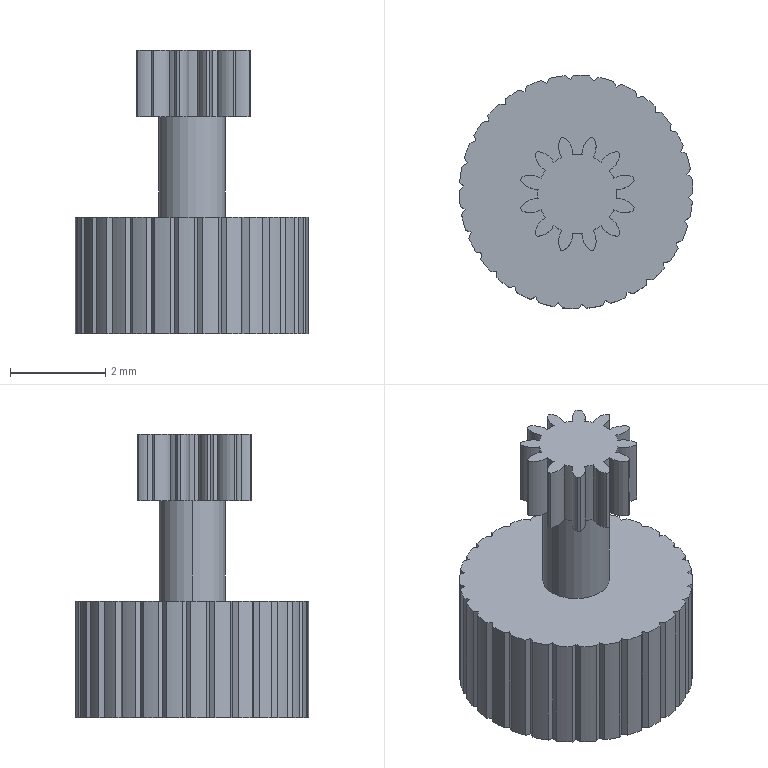Part | SolidWorks | features ICE 3, CirPattern 1, Extrusion 1, Scale 1 | 1 solid | 150 faces | box 4.9 x 4.9 x 5.95 mm | volume 53.374 mm3 | cylinder 86 | plane 64 | commonest cylinder face diameters 4.9 x31 0.84 x28 1.661 x13 2.45 x12 1.4 x2